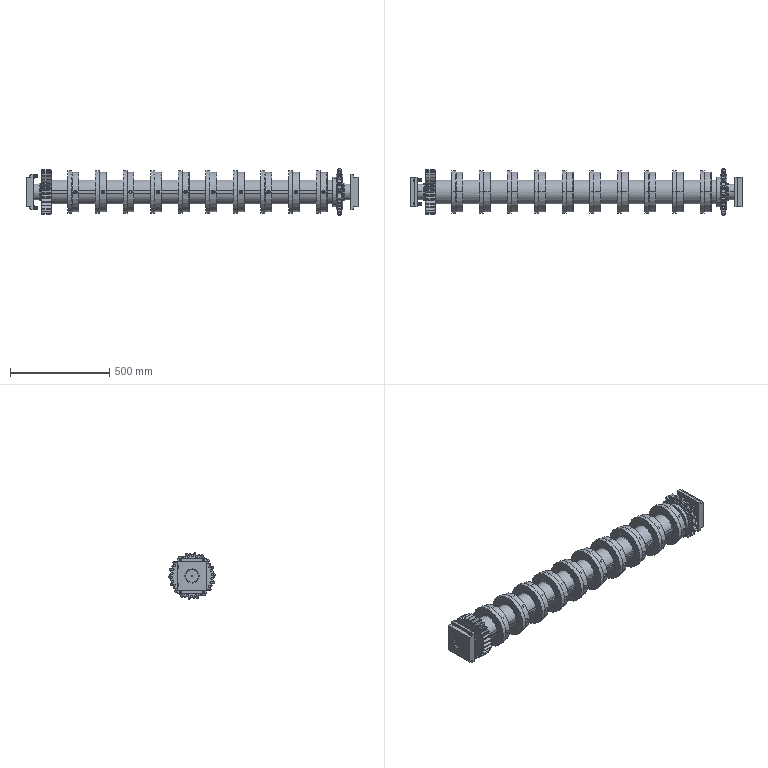Part | SolidWorks | 71 solids | 1972 faces | box 1672 x 235.877 x 235.04 mm | volume 32005063 mm3 | cylinder 851 | plane 463 | cone 352 | sphere 144 | torus 102 | spline 60 | commonest cylinder face diameters 20 x84 10.2 x80 13 x80 89.75 x66 95.25 x66 150 x42